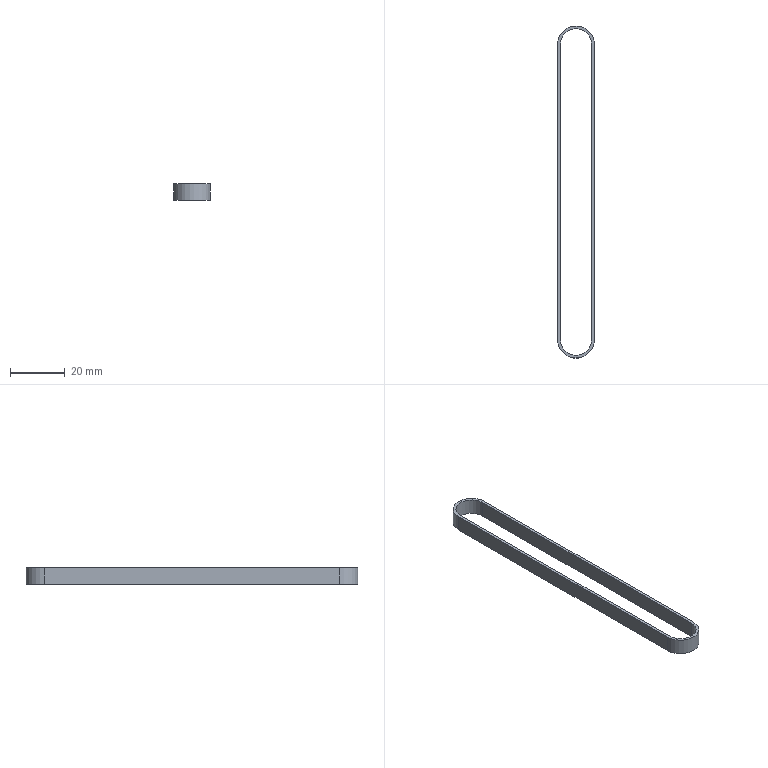Part | SolidWorks | features Extrusion 1 | 1 solid | 10 faces | box 13.5 x 121.5 x 6 mm | volume 1562 mm3 | plane 6 | cylinder 4 | commonest cylinder face diameters 11.46 x2 13.5 x2
STEP:
#1=CARTESIAN_POINT('',(-6.75,-54.,6.));
#2=VERTEX_POINT('',#1);
#3=CARTESIAN_POINT('',(6.75,-54.,6.));
#4=VERTEX_POINT('',#3);
#5=CARTESIAN_POINT('',(0.,-54.,6.));
#6=DIRECTION('',(0.,0.,1.));
#7=DIRECTION('',(1.,0.,0.));
#8=AXIS2_PLACEMENT_3D('',#5,#6,#7);
#9=CIRCLE('',#8,6.75);
#10=EDGE_CURVE('',#2,#4,#9,.T.);
#11=ORIENTED_EDGE('',*,*,#10,.T.);
#12=CARTESIAN_POINT('',(6.75,54.,6.));
#13=VERTEX_POINT('',#12);
#14=CARTESIAN_POINT('',(6.75,-54.,6.));
#15=DIRECTION('',(0.,1.,0.));
#16=VECTOR('',#15,1000.);
#17=LINE('',#14,#16);
#18=EDGE_CURVE('',#4,#13,#17,.T.);
#19=ORIENTED_EDGE('',*,*,#18,.T.);
#20=CARTESIAN_POINT('',(-6.75,54.,6.));
#21=VERTEX_POINT('',#20);
#22=CARTESIAN_POINT('',(0.,54.,6.));
#23=DIRECTION('',(0.,0.,1.));
#24=DIRECTION('',(1.,0.,0.));
#25=AXIS2_PLACEMENT_3D('',#22,#23,#24);
#26=CIRCLE('',#25,6.75);
#27=EDGE_CURVE('',#13,#21,#26,.T.);
#28=ORIENTED_EDGE('',*,*,#27,.T.);
#29=CARTESIAN_POINT('',(-6.75,-54.,6.));
#30=DIRECTION('',(0.,-1.,0.));
#31=VECTOR('',#30,1000.);
#32=LINE('',#29,#31);
#33=EDGE_CURVE('',#21,#2,#32,.T.);
#34=ORIENTED_EDGE('',*,*,#33,.T.);
#35=EDGE_LOOP('',(#11,#19,#28,#34));
#36=FACE_OUTER_BOUND('',#35,.T.);
#37=CARTESIAN_POINT('',(5.73,-54.,6.));
#38=VERTEX_POINT('',#37);
#39=CARTESIAN_POINT('',(5.73,54.,6.));
#40=VERTEX_POINT('',#39);
#41=CARTESIAN_POINT('',(5.73,-54.,6.));
#42=DIRECTION('',(0.,1.,0.));
#43=VECTOR('',#42,1000.);
#44=LINE('',#41,#43);
#45=EDGE_CURVE('',#38,#40,#44,.T.);
#46=ORIENTED_EDGE('',*,*,#45,.F.);
#47=CARTESIAN_POINT('',(-5.73,-54.,6.));
#48=VERTEX_POINT('',#47);
#49=CARTESIAN_POINT('',(0.,-54.,6.));
#50=DIRECTION('',(0.,0.,1.));
#51=DIRECTION('',(1.,0.,0.));
#52=AXIS2_PLACEMENT_3D('',#49,#50,#51);
#53=CIRCLE('',#52,5.73);
#54=EDGE_CURVE('',#48,#38,#53,.T.);
#55=ORIENTED_EDGE('',*,*,#54,.F.);
#56=CARTESIAN_POINT('',(-5.73,54.,6.));
#57=VERTEX_POINT('',#56);
#58=CARTESIAN_POINT('',(-5.73,-54.,6.));
#59=DIRECTION('',(0.,-1.,0.));
#60=VECTOR('',#59,1000.);
#61=LINE('',#58,#60);
#62=EDGE_CURVE('',#57,#48,#61,.T.);
#63=ORIENTED_EDGE('',*,*,#62,.F.);
#64=CARTESIAN_POINT('',(0.,54.,6.));
#65=DIRECTION('',(0.,0.,1.));
#66=DIRECTION('',(1.,0.,0.));
#67=AXIS2_PLACEMENT_3D('',#64,#65,#66);
#68=CIRCLE('',#67,5.73);
#69=EDGE_CURVE('',#40,#57,#68,.T.);
#70=ORIENTED_EDGE('',*,*,#69,.F.);
#71=EDGE_LOOP('',(#46,#55,#63,#70));
#72=FACE_BOUND('',#71,.T.);
#73=CARTESIAN_POINT('',(0.,-54.,6.));
#74=DIRECTION('',(0.,0.,1.));
#75=DIRECTION('',(1.,0.,0.));
#76=AXIS2_PLACEMENT_3D('',#73,#74,#75);
#77=PLANE('',#76);
#78=ADVANCED_FACE('',(#36,#72),#77,.T.);
#79=CARTESIAN_POINT('',(-6.75,-54.,0.));
#80=VERTEX_POINT('',#79);
#81=CARTESIAN_POINT('',(6.75,-54.,0.));
#82=VERTEX_POINT('',#81);
#83=CARTESIAN_POINT('',(0.,-54.,0.));
#84=DIRECTION('',(0.,0.,1.));
#85=DIRECTION('',(1.,0.,0.));
#86=AXIS2_PLACEMENT_3D('',#83,#84,#85);
#87=CIRCLE('',#86,6.75);
#88=EDGE_CURVE('',#80,#82,#87,.T.);
#89=ORIENTED_EDGE('',*,*,#88,.F.);
#90=CARTESIAN_POINT('',(-6.75,54.,0.));
#91=VERTEX_POINT('',#90);
#92=CARTESIAN_POINT('',(-6.75,-54.,0.));
#93=DIRECTION('',(0.,-1.,0.));
#94=VECTOR('',#93,1000.);
#95=LINE('',#92,#94);
#96=EDGE_CURVE('',#91,#80,#95,.T.);
#97=ORIENTED_EDGE('',*,*,#96,.F.);
#98=CARTESIAN_POINT('',(6.75,54.,0.));
#99=VERTEX_POINT('',#98);
#100=CARTESIAN_POINT('',(0.,54.,0.));
#101=DIRECTION('',(0.,0.,1.));
#102=DIRECTION('',(1.,0.,0.));
#103=AXIS2_PLACEMENT_3D('',#100,#101,#102);
#104=CIRCLE('',#103,6.75);
#105=EDGE_CURVE('',#99,#91,#104,.T.);
#106=ORIENTED_EDGE('',*,*,#105,.F.);
#107=CARTESIAN_POINT('',(6.75,-54.,0.));
#108=DIRECTION('',(0.,1.,0.));
#109=VECTOR('',#108,1000.);
#110=LINE('',#107,#109);
#111=EDGE_CURVE('',#82,#99,#110,.T.);
#112=ORIENTED_EDGE('',*,*,#111,.F.);
#113=EDGE_LOOP('',(#89,#97,#106,#112));
#114=FACE_OUTER_BOUND('',#113,.T.);
#115=CARTESIAN_POINT('',(-5.73,-54.,0.));
#116=VERTEX_POINT('',#115);
#117=CARTESIAN_POINT('',(5.73,-54.,0.));
#118=VERTEX_POINT('',#117);
#119=CARTESIAN_POINT('',(0.,-54.,0.));
#120=DIRECTION('',(0.,0.,1.));
#121=DIRECTION('',(1.,0.,0.));
#122=AXIS2_PLACEMENT_3D('',#119,#120,#121);
#123=CIRCLE('',#122,5.73);
#124=EDGE_CURVE('',#116,#118,#123,.T.);
#125=ORIENTED_EDGE('',*,*,#124,.T.);
#126=CARTESIAN_POINT('',(5.73,54.,0.));
#127=VERTEX_POINT('',#126);
#128=CARTESIAN_POINT('',(5.73,-54.,0.));
#129=DIRECTION('',(0.,1.,0.));
#130=VECTOR('',#129,1000.);
#131=LINE('',#128,#130);
#132=EDGE_CURVE('',#118,#127,#131,.T.);
#133=ORIENTED_EDGE('',*,*,#132,.T.);
#134=CARTESIAN_POINT('',(-5.73,54.,0.));
#135=VERTEX_POINT('',#134);
#136=CARTESIAN_POINT('',(0.,54.,0.));
#137=DIRECTION('',(0.,0.,1.));
#138=DIRECTION('',(1.,0.,0.));
#139=AXIS2_PLACEMENT_3D('',#136,#137,#138);
#140=CIRCLE('',#139,5.73);
#141=EDGE_CURVE('',#127,#135,#140,.T.);
#142=ORIENTED_EDGE('',*,*,#141,.T.);
#143=CARTESIAN_POINT('',(-5.73,-54.,0.));
#144=DIRECTION('',(0.,-1.,0.));
#145=VECTOR('',#144,1000.);
#146=LINE('',#143,#145);
#147=EDGE_CURVE('',#135,#116,#146,.T.);
#148=ORIENTED_EDGE('',*,*,#147,.T.);
#149=EDGE_LOOP('',(#125,#133,#142,#148));
#150=FACE_BOUND('',#149,.T.);
#151=CARTESIAN_POINT('',(0.,-54.,0.));
#152=DIRECTION('',(0.,0.,1.));
#153=DIRECTION('',(1.,0.,0.));
#154=AXIS2_PLACEMENT_3D('',#151,#152,#153);
#155=PLANE('',#154);
#156=ADVANCED_FACE('',(#114,#150),#155,.F.);
#157=ORIENTED_EDGE('',*,*,#88,.T.);
#158=CARTESIAN_POINT('',(6.75,-54.,6.));
#159=DIRECTION('',(0.,0.,-1.));
#160=VECTOR('',#159,1000.);
#161=LINE('',#158,#160);
#162=EDGE_CURVE('',#4,#82,#161,.T.);
#163=ORIENTED_EDGE('',*,*,#162,.F.);
#164=ORIENTED_EDGE('',*,*,#10,.F.);
#165=CARTESIAN_POINT('',(-6.75,-54.,6.));
#166=DIRECTION('',(0.,0.,-1.));
#167=VECTOR('',#166,1000.);
#168=LINE('',#165,#167);
#169=EDGE_CURVE('',#2,#80,#168,.T.);
#170=ORIENTED_EDGE('',*,*,#169,.T.);
#171=EDGE_LOOP('',(#157,#163,#164,#170));
#172=FACE_OUTER_BOUND('',#171,.T.);
#173=CARTESIAN_POINT('',(0.,-54.,6.));
#174=DIRECTION('',(0.,0.,-1.));
#175=DIRECTION('',(-1.,0.,0.));
#176=AXIS2_PLACEMENT_3D('',#173,#174,#175);
#177=CYLINDRICAL_SURFACE('',#176,6.75);
#178=ADVANCED_FACE('',(#172),#177,.T.);
#179=ORIENTED_EDGE('',*,*,#111,.T.);
#180=CARTESIAN_POINT('',(6.75,54.,6.));
#181=DIRECTION('',(0.,0.,-1.));
#182=VECTOR('',#181,1000.);
#183=LINE('',#180,#182);
#184=EDGE_CURVE('',#13,#99,#183,.T.);
#185=ORIENTED_EDGE('',*,*,#184,.F.);
#186=ORIENTED_EDGE('',*,*,#18,.F.);
#187=ORIENTED_EDGE('',*,*,#162,.T.);
#188=EDGE_LOOP('',(#179,#185,#186,#187));
#189=FACE_OUTER_BOUND('',#188,.T.);
#190=CARTESIAN_POINT('',(6.75,-54.,6.));
#191=DIRECTION('',(-1.,0.,0.));
#192=DIRECTION('',(0.,-1.,0.));
#193=AXIS2_PLACEMENT_3D('',#190,#191,#192);
#194=PLANE('',#193);
#195=ADVANCED_FACE('',(#189),#194,.F.);
#196=ORIENTED_EDGE('',*,*,#105,.T.);
#197=CARTESIAN_POINT('',(-6.75,54.,6.));
#198=DIRECTION('',(0.,0.,-1.));
#199=VECTOR('',#198,1000.);
#200=LINE('',#197,#199);
#201=EDGE_CURVE('',#21,#91,#200,.T.);
#202=ORIENTED_EDGE('',*,*,#201,.F.);
#203=ORIENTED_EDGE('',*,*,#27,.F.);
#204=ORIENTED_EDGE('',*,*,#184,.T.);
#205=EDGE_LOOP('',(#196,#202,#203,#204));
#206=FACE_OUTER_BOUND('',#205,.T.);
#207=CARTESIAN_POINT('',(0.,54.,6.));
#208=DIRECTION('',(0.,0.,-1.));
#209=DIRECTION('',(-1.,0.,0.));
#210=AXIS2_PLACEMENT_3D('',#207,#208,#209);
#211=CYLINDRICAL_SURFACE('',#210,6.75);
#212=ADVANCED_FACE('',(#206),#211,.T.);
#213=ORIENTED_EDGE('',*,*,#96,.T.);
#214=ORIENTED_EDGE('',*,*,#169,.F.);
#215=ORIENTED_EDGE('',*,*,#33,.F.);
#216=ORIENTED_EDGE('',*,*,#201,.T.);
#217=EDGE_LOOP('',(#213,#214,#215,#216));
#218=FACE_OUTER_BOUND('',#217,.T.);
#219=CARTESIAN_POINT('',(-6.75,-54.,6.));
#220=DIRECTION('',(1.,0.,0.));
#221=DIRECTION('',(0.,1.,0.));
#222=AXIS2_PLACEMENT_3D('',#219,#220,#221);
#223=PLANE('',#222);
#224=ADVANCED_FACE('',(#218),#223,.F.);
#225=ORIENTED_EDGE('',*,*,#124,.F.);
#226=CARTESIAN_POINT('',(-5.73,-54.,6.));
#227=DIRECTION('',(0.,0.,-1.));
#228=VECTOR('',#227,1000.);
#229=LINE('',#226,#228);
#230=EDGE_CURVE('',#48,#116,#229,.T.);
#231=ORIENTED_EDGE('',*,*,#230,.F.);
#232=ORIENTED_EDGE('',*,*,#54,.T.);
#233=CARTESIAN_POINT('',(5.73,-54.,6.));
#234=DIRECTION('',(0.,0.,-1.));
#235=VECTOR('',#234,1000.);
#236=LINE('',#233,#235);
#237=EDGE_CURVE('',#38,#118,#236,.T.);
#238=ORIENTED_EDGE('',*,*,#237,.T.);
#239=EDGE_LOOP('',(#225,#231,#232,#238));
#240=FACE_OUTER_BOUND('',#239,.T.);
#241=CARTESIAN_POINT('',(0.,-54.,6.));
#242=DIRECTION('',(0.,0.,-1.));
#243=DIRECTION('',(-1.,0.,0.));
#244=AXIS2_PLACEMENT_3D('',#241,#242,#243);
#245=CYLINDRICAL_SURFACE('',#244,5.73);
#246=ADVANCED_FACE('',(#240),#245,.F.);
#247=ORIENTED_EDGE('',*,*,#132,.F.);
#248=ORIENTED_EDGE('',*,*,#237,.F.);
#249=ORIENTED_EDGE('',*,*,#45,.T.);
#250=CARTESIAN_POINT('',(5.73,54.,6.));
#251=DIRECTION('',(0.,0.,-1.));
#252=VECTOR('',#251,1000.);
#253=LINE('',#250,#252);
#254=EDGE_CURVE('',#40,#127,#253,.T.);
#255=ORIENTED_EDGE('',*,*,#254,.T.);
#256=EDGE_LOOP('',(#247,#248,#249,#255));
#257=FACE_OUTER_BOUND('',#256,.T.);
#258=CARTESIAN_POINT('',(5.73,-54.,6.));
#259=DIRECTION('',(-1.,0.,0.));
#260=DIRECTION('',(0.,-1.,0.));
#261=AXIS2_PLACEMENT_3D('',#258,#259,#260);
#262=PLANE('',#261);
#263=ADVANCED_FACE('',(#257),#262,.T.);
#264=ORIENTED_EDGE('',*,*,#141,.F.);
#265=ORIENTED_EDGE('',*,*,#254,.F.);
#266=ORIENTED_EDGE('',*,*,#69,.T.);
#267=CARTESIAN_POINT('',(-5.73,54.,6.));
#268=DIRECTION('',(0.,0.,-1.));
#269=VECTOR('',#268,1000.);
#270=LINE('',#267,#269);
#271=EDGE_CURVE('',#57,#135,#270,.T.);
#272=ORIENTED_EDGE('',*,*,#271,.T.);
#273=EDGE_LOOP('',(#264,#265,#266,#272));
#274=FACE_OUTER_BOUND('',#273,.T.);
#275=CARTESIAN_POINT('',(0.,54.,6.));
#276=DIRECTION('',(0.,0.,-1.));
#277=DIRECTION('',(-1.,0.,0.));
#278=AXIS2_PLACEMENT_3D('',#275,#276,#277);
#279=CYLINDRICAL_SURFACE('',#278,5.73);
#280=ADVANCED_FACE('',(#274),#279,.F.);
#281=ORIENTED_EDGE('',*,*,#147,.F.);
#282=ORIENTED_EDGE('',*,*,#271,.F.);
#283=ORIENTED_EDGE('',*,*,#62,.T.);
#284=ORIENTED_EDGE('',*,*,#230,.T.);
#285=EDGE_LOOP('',(#281,#282,#283,#284));
#286=FACE_OUTER_BOUND('',#285,.T.);
#287=CARTESIAN_POINT('',(-5.73,-54.,6.));
#288=DIRECTION('',(1.,0.,0.));
#289=DIRECTION('',(0.,1.,0.));
#290=AXIS2_PLACEMENT_3D('',#287,#288,#289);
#291=PLANE('',#290);
#292=ADVANCED_FACE('',(#286),#291,.T.);
#293=CLOSED_SHELL('',(#78,#156,#178,#195,#212,#224,#246,#263,#280,#292));
#294=MANIFOLD_SOLID_BREP('',#293);
#295=CARTESIAN_POINT('',(0.,0.,0.));
#296=DIRECTION('',(0.,0.,1.));
#297=DIRECTION('',(1.,0.,0.));
#298=AXIS2_PLACEMENT_3D('',#295,#296,#297);
#299=(LENGTH_UNIT()NAMED_UNIT(*)SI_UNIT(.MILLI.,.METRE.));
#300=UNCERTAINTY_MEASURE_WITH_UNIT(LENGTH_MEASURE(0.00001),#299,'','');
#301=(NAMED_UNIT(*)PLANE_ANGLE_UNIT()SI_UNIT($,.RADIAN.));
#302=(NAMED_UNIT(*)SI_UNIT($,.STERADIAN.)SOLID_ANGLE_UNIT());
#303=(GEOMETRIC_REPRESENTATION_CONTEXT(3)GLOBAL_UNCERTAINTY_ASSIGNED_CONTEXT((#300))GLOBAL_UNIT_ASSIGNED_CONTEXT((#299,#301,#302))REPRESENTATION_CONTEXT('',''));
#304=ADVANCED_BREP_SHAPE_REPRESENTATION('',(#294,#298),#303);